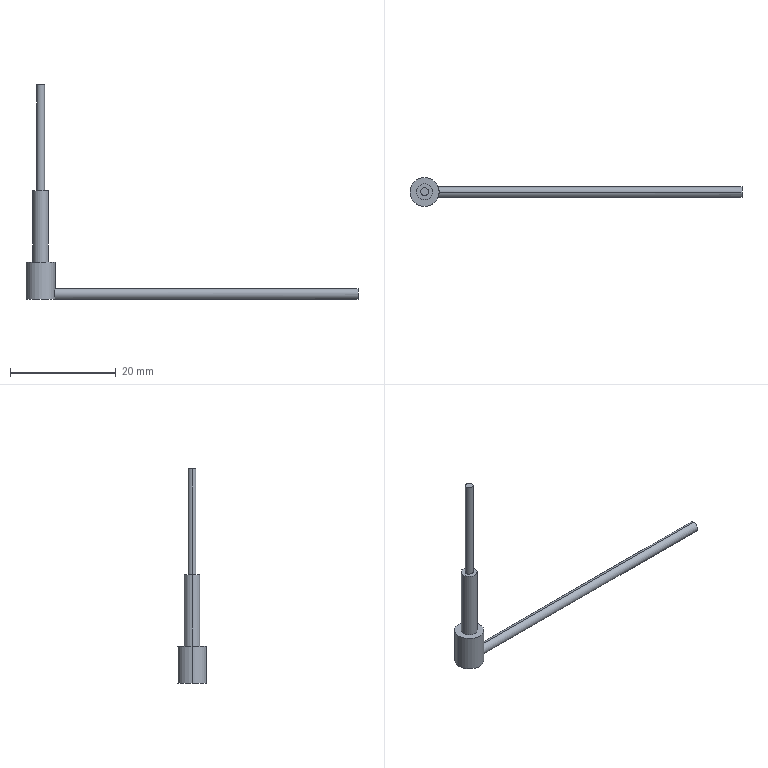Part | SolidWorks | features BaseBody 2 | 2 solids | 14 faces | box 62.75 x 5.5 x 40.5 mm | volume 476.928 mm3 | cylinder 8 | plane 6 | commonest cylinder face diameters 1.5 x2 2 x2 3 x2 5.5 x2
STEP:
#1=CARTESIAN_POINT('',(-0.75,0.,20.5));
#2=VERTEX_POINT('',#1);
#3=CARTESIAN_POINT('',(0.75,0.,20.5));
#4=VERTEX_POINT('',#3);
#5=CARTESIAN_POINT('',(0.,0.,20.5));
#6=DIRECTION('',(0.,0.,1.));
#7=DIRECTION('',(1.,0.,0.));
#8=AXIS2_PLACEMENT_3D('',#5,#6,#7);
#9=CIRCLE('',#8,0.75);
#10=EDGE_CURVE('',#2,#4,#9,.T.);
#11=ORIENTED_EDGE('',*,*,#10,.F.);
#12=CARTESIAN_POINT('',(0.,0.,20.5));
#13=DIRECTION('',(0.,0.,1.));
#14=DIRECTION('',(1.,0.,0.));
#15=AXIS2_PLACEMENT_3D('',#12,#13,#14);
#16=CIRCLE('',#15,0.75);
#17=EDGE_CURVE('',#4,#2,#16,.T.);
#18=ORIENTED_EDGE('',*,*,#17,.F.);
#19=EDGE_LOOP('',(#11,#18));
#20=FACE_OUTER_BOUND('',#19,.T.);
#21=CARTESIAN_POINT('',(0.,0.,20.5));
#22=DIRECTION('',(0.,0.,1.));
#23=DIRECTION('',(1.,0.,0.));
#24=AXIS2_PLACEMENT_3D('',#21,#22,#23);
#25=PLANE('',#24);
#26=ADVANCED_FACE('',(#20),#25,.F.);
#27=CARTESIAN_POINT('',(-0.75,0.,40.5));
#28=VERTEX_POINT('',#27);
#29=CARTESIAN_POINT('',(0.75,0.,40.5));
#30=VERTEX_POINT('',#29);
#31=CARTESIAN_POINT('',(0.,0.,40.5));
#32=DIRECTION('',(0.,0.,1.));
#33=DIRECTION('',(1.,0.,0.));
#34=AXIS2_PLACEMENT_3D('',#31,#32,#33);
#35=CIRCLE('',#34,0.75);
#36=EDGE_CURVE('',#28,#30,#35,.T.);
#37=ORIENTED_EDGE('',*,*,#36,.T.);
#38=CARTESIAN_POINT('',(0.,0.,40.5));
#39=DIRECTION('',(0.,0.,1.));
#40=DIRECTION('',(1.,0.,0.));
#41=AXIS2_PLACEMENT_3D('',#38,#39,#40);
#42=CIRCLE('',#41,0.75);
#43=EDGE_CURVE('',#30,#28,#42,.T.);
#44=ORIENTED_EDGE('',*,*,#43,.T.);
#45=EDGE_LOOP('',(#37,#44));
#46=FACE_OUTER_BOUND('',#45,.T.);
#47=CARTESIAN_POINT('',(0.,0.,40.5));
#48=DIRECTION('',(0.,0.,1.));
#49=DIRECTION('',(1.,0.,0.));
#50=AXIS2_PLACEMENT_3D('',#47,#48,#49);
#51=PLANE('',#50);
#52=ADVANCED_FACE('',(#46),#51,.T.);
#53=CARTESIAN_POINT('',(0.75,0.,40.5));
#54=DIRECTION('',(0.,0.,-1.));
#55=VECTOR('',#54,1000.);
#56=LINE('',#53,#55);
#57=EDGE_CURVE('',#30,#4,#56,.T.);
#58=ORIENTED_EDGE('',*,*,#57,.F.);
#59=ORIENTED_EDGE('',*,*,#36,.F.);
#60=CARTESIAN_POINT('',(-0.75,0.,40.5));
#61=DIRECTION('',(0.,0.,-1.));
#62=VECTOR('',#61,1000.);
#63=LINE('',#60,#62);
#64=EDGE_CURVE('',#28,#2,#63,.T.);
#65=ORIENTED_EDGE('',*,*,#64,.T.);
#66=ORIENTED_EDGE('',*,*,#10,.T.);
#67=EDGE_LOOP('',(#58,#59,#65,#66));
#68=FACE_OUTER_BOUND('',#67,.T.);
#69=CARTESIAN_POINT('',(0.,0.,40.5));
#70=DIRECTION('',(0.,0.,-1.));
#71=DIRECTION('',(-1.,0.,0.));
#72=AXIS2_PLACEMENT_3D('',#69,#70,#71);
#73=CYLINDRICAL_SURFACE('',#72,0.75);
#74=ADVANCED_FACE('',(#68),#73,.T.);
#75=ORIENTED_EDGE('',*,*,#43,.F.);
#76=ORIENTED_EDGE('',*,*,#57,.T.);
#77=ORIENTED_EDGE('',*,*,#17,.T.);
#78=ORIENTED_EDGE('',*,*,#64,.F.);
#79=EDGE_LOOP('',(#75,#76,#77,#78));
#80=FACE_OUTER_BOUND('',#79,.T.);
#81=CARTESIAN_POINT('',(0.,0.,40.5));
#82=DIRECTION('',(0.,0.,-1.));
#83=DIRECTION('',(-1.,0.,0.));
#84=AXIS2_PLACEMENT_3D('',#81,#82,#83);
#85=CYLINDRICAL_SURFACE('',#84,0.75);
#86=ADVANCED_FACE('',(#80),#85,.T.);
#87=CLOSED_SHELL('',(#26,#52,#74,#86));
#88=MANIFOLD_SOLID_BREP('',#87);
#89=CARTESIAN_POINT('',(60.,0.,2.));
#90=VERTEX_POINT('',#89);
#91=CARTESIAN_POINT('',(60.,0.,0.));
#92=VERTEX_POINT('',#91);
#93=CARTESIAN_POINT('',(60.,0.,1.));
#94=DIRECTION('',(1.,0.,0.));
#95=DIRECTION('',(0.,0.,-1.));
#96=AXIS2_PLACEMENT_3D('',#93,#94,#95);
#97=CIRCLE('',#96,1.);
#98=EDGE_CURVE('',#90,#92,#97,.T.);
#99=ORIENTED_EDGE('',*,*,#98,.T.);
#100=CARTESIAN_POINT('',(60.,0.,1.));
#101=DIRECTION('',(1.,0.,0.));
#102=DIRECTION('',(0.,0.,-1.));
#103=AXIS2_PLACEMENT_3D('',#100,#101,#102);
#104=CIRCLE('',#103,1.);
#105=EDGE_CURVE('',#92,#90,#104,.T.);
#106=ORIENTED_EDGE('',*,*,#105,.T.);
#107=EDGE_LOOP('',(#99,#106));
#108=FACE_OUTER_BOUND('',#107,.T.);
#109=CARTESIAN_POINT('',(60.,0.,1.));
#110=DIRECTION('',(1.,0.,0.));
#111=DIRECTION('',(0.,1.,0.));
#112=AXIS2_PLACEMENT_3D('',#109,#110,#111);
#113=PLANE('',#112);
#114=ADVANCED_FACE('',(#108),#113,.T.);
#115=CARTESIAN_POINT('',(2.75,0.,0.));
#116=VERTEX_POINT('',#115);
#117=CARTESIAN_POINT('',(60.,0.,0.));
#118=DIRECTION('',(-1.,0.,0.));
#119=VECTOR('',#118,1000.);
#120=LINE('',#117,#119);
#121=EDGE_CURVE('',#92,#116,#120,.T.);
#122=ORIENTED_EDGE('',*,*,#121,.F.);
#123=ORIENTED_EDGE('',*,*,#98,.F.);
#124=CARTESIAN_POINT('',(2.75,0.,2.));
#125=VERTEX_POINT('',#124);
#126=CARTESIAN_POINT('',(60.,0.,2.));
#127=DIRECTION('',(-1.,0.,0.));
#128=VECTOR('',#127,1000.);
#129=LINE('',#126,#128);
#130=EDGE_CURVE('',#90,#125,#129,.T.);
#131=ORIENTED_EDGE('',*,*,#130,.T.);
#132=CARTESIAN_POINT('',(2.75,0.,2.));
#133=CARTESIAN_POINT('',(2.75,-0.0625,2.));
#134=CARTESIAN_POINT('',(2.748,-0.1267,1.994));
#135=CARTESIAN_POINT('',(2.741,-0.2236,1.975));
#136=CARTESIAN_POINT('',(2.738,-0.256,1.967));
#137=CARTESIAN_POINT('',(2.733,-0.3044,1.953));
#138=CARTESIAN_POINT('',(2.73,-0.3286,1.945));
#139=CARTESIAN_POINT('',(2.727,-0.3567,1.934));
#140=CARTESIAN_POINT('',(2.725,-0.3687,1.93));
#141=CARTESIAN_POINT('',(2.724,-0.3767,1.926));
#142=CARTESIAN_POINT('',(2.723,-0.382,1.924));
#143=CARTESIAN_POINT('',(2.717,-0.4276,1.905));
#144=CARTESIAN_POINT('',(2.708,-0.478,1.881));
#145=CARTESIAN_POINT('',(2.692,-0.5607,1.829));
#146=CARTESIAN_POINT('',(2.686,-0.5895,1.809));
#147=CARTESIAN_POINT('',(2.676,-0.6334,1.774));
#148=CARTESIAN_POINT('',(2.672,-0.6481,1.762));
#149=CARTESIAN_POINT('',(2.665,-0.6778,1.736));
#150=CARTESIAN_POINT('',(2.662,-0.6917,1.723));
#151=CARTESIAN_POINT('',(2.641,-0.7708,1.643));
#152=CARTESIAN_POINT('',(2.628,-0.8127,1.585));
#153=CARTESIAN_POINT('',(2.616,-0.8483,1.53));
#154=CARTESIAN_POINT('',(2.614,-0.8546,1.519));
#155=CARTESIAN_POINT('',(2.612,-0.8615,1.508));
#156=CARTESIAN_POINT('',(2.611,-0.8629,1.505));
#157=CARTESIAN_POINT('',(2.61,-0.8655,1.501));
#158=CARTESIAN_POINT('',(2.61,-0.8676,1.497));
#159=CARTESIAN_POINT('',(2.607,-0.874,1.486));
#160=CARTESIAN_POINT('',(2.603,-0.8863,1.464));
#161=CARTESIAN_POINT('',(2.599,-0.8974,1.442));
#162=CARTESIAN_POINT('',(2.595,-0.9111,1.412));
#163=CARTESIAN_POINT('',(2.593,-0.9166,1.4));
#164=CARTESIAN_POINT('',(2.571,-0.9769,1.255));
#165=CARTESIAN_POINT('',(2.562,-1.,1.123));
#166=CARTESIAN_POINT('',(2.562,-1.,0.9379));
#167=CARTESIAN_POINT('',(2.564,-0.9942,0.8741));
#168=CARTESIAN_POINT('',(2.571,-0.9754,0.7773));
#169=CARTESIAN_POINT('',(2.574,-0.9675,0.7448));
#170=CARTESIAN_POINT('',(2.58,-0.9529,0.6961));
#171=CARTESIAN_POINT('',(2.583,-0.9449,0.6717));
#172=CARTESIAN_POINT('',(2.586,-0.9343,0.6434));
#173=CARTESIAN_POINT('',(2.588,-0.9296,0.6313));
#174=CARTESIAN_POINT('',(2.589,-0.9263,0.6232));
#175=CARTESIAN_POINT('',(2.59,-0.924,0.6176));
#176=CARTESIAN_POINT('',(2.596,-0.9069,0.5766));
#177=CARTESIAN_POINT('',(2.605,-0.8841,0.5281));
#178=CARTESIAN_POINT('',(2.621,-0.8326,0.4452));
#179=CARTESIAN_POINT('',(2.628,-0.8126,0.4159));
#180=CARTESIAN_POINT('',(2.638,-0.7772,0.3704));
#181=CARTESIAN_POINT('',(2.642,-0.7645,0.3551));
#182=CARTESIAN_POINT('',(2.649,-0.7372,0.3241));
#183=CARTESIAN_POINT('',(2.654,-0.7218,0.3076));
#184=CARTESIAN_POINT('',(2.673,-0.6478,0.2336));
#185=CARTESIAN_POINT('',(2.687,-0.588,0.1886));
#186=CARTESIAN_POINT('',(2.703,-0.5054,0.1365));
#187=CARTESIAN_POINT('',(2.708,-0.479,0.1218));
#188=CARTESIAN_POINT('',(2.714,-0.4417,0.1027));
#189=CARTESIAN_POINT('',(2.717,-0.4237,0.09403));
#190=CARTESIAN_POINT('',(2.72,-0.4037,0.08508));
#191=CARTESIAN_POINT('',(2.721,-0.3954,0.08149));
#192=CARTESIAN_POINT('',(2.722,-0.3899,0.07915));
#193=CARTESIAN_POINT('',(2.722,-0.3885,0.07855));
#194=CARTESIAN_POINT('',(2.741,-0.257,0.02376));
#195=CARTESIAN_POINT('',(2.75,-0.125,0.));
#196=CARTESIAN_POINT('',(2.75,0.,0.));
#197=B_SPLINE_CURVE_WITH_KNOTS('',3,(#132,#133,#134,#135,#136,#137,#138,#139,#140,#141,#142,#143,#144,#145,#146,#147,#148,#149,#150,#151,#152,#153,#154,#155,#156,#157,#158,#159,#160,#161,#162,#163,#164,#165,#166,#167,#168,#169,#170,#171,#172,#173,#174,#175,#176,#177,#178,#179,#180,#181,#182,#183,#184,#185,#186,#187,#188,#189,#190,#191,#192,#193,#194,#195,#196),.UNSPECIFIED.,.F.,.F.,(4,2,2,1,1,2,2,2,2,2,2,2,2,2,2,1,2,2,2,2,2,1,1,2,2,2,2,2,2,2,2,1,1,2,2,4),(0.,0.0625,0.09375,0.1094,0.1172,0.1211,0.125,0.1875,0.2187,0.2344,0.25,0.3125,0.3281,0.332,0.3359,0.3437,0.3594,0.375,0.5,0.5625,0.5937,0.6094,0.6172,0.6211,0.625,0.6875,0.7187,0.7344,0.75,0.8125,0.8437,0.8594,0.8672,0.8711,0.875,1.),.UNSPECIFIED.);
#198=EDGE_CURVE('',#125,#116,#197,.T.);
#199=ORIENTED_EDGE('',*,*,#198,.T.);
#200=EDGE_LOOP('',(#122,#123,#131,#199));
#201=FACE_OUTER_BOUND('',#200,.T.);
#202=CARTESIAN_POINT('',(60.,0.,1.));
#203=DIRECTION('',(-1.,0.,0.));
#204=DIRECTION('',(0.,0.,1.));
#205=AXIS2_PLACEMENT_3D('',#202,#203,#204);
#206=CYLINDRICAL_SURFACE('',#205,1.);
#207=ADVANCED_FACE('',(#201),#206,.T.);
#208=CARTESIAN_POINT('',(-1.5,0.,20.5));
#209=VERTEX_POINT('',#208);
#210=CARTESIAN_POINT('',(1.5,0.,20.5));
#211=VERTEX_POINT('',#210);
#212=CARTESIAN_POINT('',(0.,0.,20.5));
#213=DIRECTION('',(0.,0.,1.));
#214=DIRECTION('',(1.,0.,0.));
#215=AXIS2_PLACEMENT_3D('',#212,#213,#214);
#216=CIRCLE('',#215,1.5);
#217=EDGE_CURVE('',#209,#211,#216,.T.);
#218=ORIENTED_EDGE('',*,*,#217,.T.);
#219=CARTESIAN_POINT('',(0.,0.,20.5));
#220=DIRECTION('',(0.,0.,1.));
#221=DIRECTION('',(1.,0.,0.));
#222=AXIS2_PLACEMENT_3D('',#219,#220,#221);
#223=CIRCLE('',#222,1.5);
#224=EDGE_CURVE('',#211,#209,#223,.T.);
#225=ORIENTED_EDGE('',*,*,#224,.T.);
#226=EDGE_LOOP('',(#218,#225));
#227=FACE_OUTER_BOUND('',#226,.T.);
#228=CARTESIAN_POINT('',(0.,0.,20.5));
#229=DIRECTION('',(0.,0.,1.));
#230=DIRECTION('',(1.,0.,0.));
#231=AXIS2_PLACEMENT_3D('',#228,#229,#230);
#232=PLANE('',#231);
#233=ADVANCED_FACE('',(#227),#232,.T.);
#234=CARTESIAN_POINT('',(1.5,0.,7.));
#235=VERTEX_POINT('',#234);
#236=CARTESIAN_POINT('',(1.5,0.,20.5));
#237=DIRECTION('',(0.,0.,-1.));
#238=VECTOR('',#237,1000.);
#239=LINE('',#236,#238);
#240=EDGE_CURVE('',#211,#235,#239,.T.);
#241=ORIENTED_EDGE('',*,*,#240,.F.);
#242=ORIENTED_EDGE('',*,*,#217,.F.);
#243=CARTESIAN_POINT('',(-1.5,0.,7.));
#244=VERTEX_POINT('',#243);
#245=CARTESIAN_POINT('',(-1.5,0.,20.5));
#246=DIRECTION('',(0.,0.,-1.));
#247=VECTOR('',#246,1000.);
#248=LINE('',#245,#247);
#249=EDGE_CURVE('',#209,#244,#248,.T.);
#250=ORIENTED_EDGE('',*,*,#249,.T.);
#251=CARTESIAN_POINT('',(0.,0.,7.));
#252=DIRECTION('',(0.,0.,1.));
#253=DIRECTION('',(1.,0.,0.));
#254=AXIS2_PLACEMENT_3D('',#251,#252,#253);
#255=CIRCLE('',#254,1.5);
#256=EDGE_CURVE('',#244,#235,#255,.T.);
#257=ORIENTED_EDGE('',*,*,#256,.T.);
#258=EDGE_LOOP('',(#241,#242,#250,#257));
#259=FACE_OUTER_BOUND('',#258,.T.);
#260=CARTESIAN_POINT('',(0.,0.,20.5));
#261=DIRECTION('',(0.,0.,-1.));
#262=DIRECTION('',(-1.,0.,0.));
#263=AXIS2_PLACEMENT_3D('',#260,#261,#262);
#264=CYLINDRICAL_SURFACE('',#263,1.5);
#265=ADVANCED_FACE('',(#259),#264,.T.);
#266=CARTESIAN_POINT('',(-2.75,0.,0.));
#267=VERTEX_POINT('',#266);
#268=CARTESIAN_POINT('',(0.,0.,0.));
#269=DIRECTION('',(0.,0.,1.));
#270=DIRECTION('',(1.,0.,0.));
#271=AXIS2_PLACEMENT_3D('',#268,#269,#270);
#272=CIRCLE('',#271,2.75);
#273=EDGE_CURVE('',#116,#267,#272,.T.);
#274=ORIENTED_EDGE('',*,*,#273,.F.);
#275=CARTESIAN_POINT('',(0.,0.,0.));
#276=DIRECTION('',(0.,0.,1.));
#277=DIRECTION('',(1.,0.,0.));
#278=AXIS2_PLACEMENT_3D('',#275,#276,#277);
#279=CIRCLE('',#278,2.75);
#280=EDGE_CURVE('',#267,#116,#279,.T.);
#281=ORIENTED_EDGE('',*,*,#280,.F.);
#282=EDGE_LOOP('',(#274,#281));
#283=FACE_OUTER_BOUND('',#282,.T.);
#284=CARTESIAN_POINT('',(0.,0.,0.));
#285=DIRECTION('',(0.,0.,1.));
#286=DIRECTION('',(1.,0.,0.));
#287=AXIS2_PLACEMENT_3D('',#284,#285,#286);
#288=PLANE('',#287);
#289=ADVANCED_FACE('',(#283),#288,.F.);
#290=ORIENTED_EDGE('',*,*,#256,.F.);
#291=CARTESIAN_POINT('',(0.,0.,7.));
#292=DIRECTION('',(0.,0.,1.));
#293=DIRECTION('',(1.,0.,0.));
#294=AXIS2_PLACEMENT_3D('',#291,#292,#293);
#295=CIRCLE('',#294,1.5);
#296=EDGE_CURVE('',#235,#244,#295,.T.);
#297=ORIENTED_EDGE('',*,*,#296,.F.);
#298=EDGE_LOOP('',(#290,#297));
#299=FACE_BOUND('',#298,.T.);
#300=CARTESIAN_POINT('',(-2.75,0.,7.));
#301=VERTEX_POINT('',#300);
#302=CARTESIAN_POINT('',(2.75,0.,7.));
#303=VERTEX_POINT('',#302);
#304=CARTESIAN_POINT('',(0.,0.,7.));
#305=DIRECTION('',(0.,0.,1.));
#306=DIRECTION('',(1.,0.,0.));
#307=AXIS2_PLACEMENT_3D('',#304,#305,#306);
#308=CIRCLE('',#307,2.75);
#309=EDGE_CURVE('',#301,#303,#308,.T.);
#310=ORIENTED_EDGE('',*,*,#309,.T.);
#311=CARTESIAN_POINT('',(0.,0.,7.));
#312=DIRECTION('',(0.,0.,1.));
#313=DIRECTION('',(1.,0.,0.));
#314=AXIS2_PLACEMENT_3D('',#311,#312,#313);
#315=CIRCLE('',#314,2.75);
#316=EDGE_CURVE('',#303,#301,#315,.T.);
#317=ORIENTED_EDGE('',*,*,#316,.T.);
#318=EDGE_LOOP('',(#310,#317));
#319=FACE_OUTER_BOUND('',#318,.T.);
#320=CARTESIAN_POINT('',(0.,0.,7.));
#321=DIRECTION('',(0.,0.,1.));
#322=DIRECTION('',(1.,0.,0.));
#323=AXIS2_PLACEMENT_3D('',#320,#321,#322);
#324=PLANE('',#323);
#325=ADVANCED_FACE('',(#299,#319),#324,.T.);
#326=CARTESIAN_POINT('',(2.75,0.,7.));
#327=DIRECTION('',(0.,0.,-1.));
#328=VECTOR('',#327,1000.);
#329=LINE('',#326,#328);
#330=EDGE_CURVE('',#303,#125,#329,.T.);
#331=ORIENTED_EDGE('',*,*,#330,.F.);
#332=ORIENTED_EDGE('',*,*,#309,.F.);
#333=CARTESIAN_POINT('',(-2.75,0.,7.));
#334=DIRECTION('',(0.,0.,-1.));
#335=VECTOR('',#334,1000.);
#336=LINE('',#333,#335);
#337=EDGE_CURVE('',#301,#267,#336,.T.);
#338=ORIENTED_EDGE('',*,*,#337,.T.);
#339=ORIENTED_EDGE('',*,*,#280,.T.);
#340=ORIENTED_EDGE('',*,*,#198,.F.);
#341=EDGE_LOOP('',(#331,#332,#338,#339,#340));
#342=FACE_OUTER_BOUND('',#341,.T.);
#343=CARTESIAN_POINT('',(0.,0.,7.));
#344=DIRECTION('',(0.,0.,-1.));
#345=DIRECTION('',(-1.,0.,0.));
#346=AXIS2_PLACEMENT_3D('',#343,#344,#345);
#347=CYLINDRICAL_SURFACE('',#346,2.75);
#348=ADVANCED_FACE('',(#342),#347,.T.);
#349=ORIENTED_EDGE('',*,*,#316,.F.);
#350=ORIENTED_EDGE('',*,*,#330,.T.);
#351=CARTESIAN_POINT('',(2.75,0.,0.));
#352=CARTESIAN_POINT('',(2.75,0.06255,0.));
#353=CARTESIAN_POINT('',(2.748,0.1268,0.005887));
#354=CARTESIAN_POINT('',(2.741,0.2238,0.02481));
#355=CARTESIAN_POINT('',(2.738,0.2562,0.03279));
#356=CARTESIAN_POINT('',(2.733,0.3047,0.04741));
#357=CARTESIAN_POINT('',(2.73,0.3289,0.05537));
#358=CARTESIAN_POINT('',(2.727,0.357,0.06584));
#359=CARTESIAN_POINT('',(2.725,0.3691,0.07059));
#360=CARTESIAN_POINT('',(2.724,0.3771,0.0738));
#361=CARTESIAN_POINT('',(2.723,0.3824,0.07599));
#362=CARTESIAN_POINT('',(2.717,0.4279,0.09498));
#363=CARTESIAN_POINT('',(2.708,0.4783,0.1194));
#364=CARTESIAN_POINT('',(2.692,0.5609,0.1715));
#365=CARTESIAN_POINT('',(2.686,0.5896,0.1914));
#366=CARTESIAN_POINT('',(2.673,0.6481,0.2375));
#367=CARTESIAN_POINT('',(2.666,0.6763,0.2621));
#368=CARTESIAN_POINT('',(2.641,0.7698,0.3557));
#369=CARTESIAN_POINT('',(2.627,0.8156,0.4178));
#370=CARTESIAN_POINT('',(2.61,0.867,0.5006));
#371=CARTESIAN_POINT('',(2.605,0.8813,0.5266));
#372=CARTESIAN_POINT('',(2.599,0.8993,0.5624));
#373=CARTESIAN_POINT('',(2.596,0.9074,0.5795));
#374=CARTESIAN_POINT('',(2.593,0.9156,0.5979));
#375=CARTESIAN_POINT('',(2.592,0.9189,0.6055));
#376=CARTESIAN_POINT('',(2.591,0.921,0.6105));
#377=CARTESIAN_POINT('',(2.591,0.9214,0.6113));
#378=CARTESIAN_POINT('',(2.571,0.9767,0.7441));
#379=CARTESIAN_POINT('',(2.562,0.9999,0.8758));
#380=CARTESIAN_POINT('',(2.562,1.,1.061));
#381=CARTESIAN_POINT('',(2.564,0.9943,1.125));
#382=CARTESIAN_POINT('',(2.571,0.9756,1.222));
#383=CARTESIAN_POINT('',(2.574,0.9676,1.255));
#384=CARTESIAN_POINT('',(2.58,0.953,1.303));
#385=CARTESIAN_POINT('',(2.582,0.9477,1.32));
#386=CARTESIAN_POINT('',(2.586,0.9361,1.352));
#387=CARTESIAN_POINT('',(2.588,0.929,1.37));
#388=CARTESIAN_POINT('',(2.595,0.9113,1.413));
#389=CARTESIAN_POINT('',(2.599,0.8976,1.442));
#390=CARTESIAN_POINT('',(2.606,0.8776,1.479));
#391=CARTESIAN_POINT('',(2.608,0.8735,1.487));
#392=CARTESIAN_POINT('',(2.61,0.8671,1.498));
#393=CARTESIAN_POINT('',(2.61,0.8649,1.502));
#394=CARTESIAN_POINT('',(2.611,0.8623,1.506));
#395=CARTESIAN_POINT('',(2.614,0.8556,1.518));
#396=CARTESIAN_POINT('',(2.616,0.8478,1.53));
#397=CARTESIAN_POINT('',(2.623,0.8265,1.564));
#398=CARTESIAN_POINT('',(2.629,0.8089,1.589));
#399=CARTESIAN_POINT('',(2.638,0.7759,1.631));
#400=CARTESIAN_POINT('',(2.642,0.7638,1.646));
#401=CARTESIAN_POINT('',(2.649,0.7372,1.676));
#402=CARTESIAN_POINT('',(2.654,0.7216,1.693));
#403=CARTESIAN_POINT('',(2.673,0.6477,1.767));
#404=CARTESIAN_POINT('',(2.687,0.5879,1.812));
#405=CARTESIAN_POINT('',(2.703,0.5053,1.864));
#406=CARTESIAN_POINT('',(2.708,0.4789,1.878));
#407=CARTESIAN_POINT('',(2.714,0.4416,1.897));
#408=CARTESIAN_POINT('',(2.717,0.4235,1.906));
#409=CARTESIAN_POINT('',(2.72,0.4035,1.915));
#410=CARTESIAN_POINT('',(2.721,0.3952,1.919));
#411=CARTESIAN_POINT('',(2.722,0.3897,1.921));
#412=CARTESIAN_POINT('',(2.722,0.3883,1.922));
#413=CARTESIAN_POINT('',(2.741,0.2569,1.976));
#414=CARTESIAN_POINT('',(2.75,0.1249,2.));
#415=CARTESIAN_POINT('',(2.75,0.,2.));
#416=B_SPLINE_CURVE_WITH_KNOTS('',3,(#351,#352,#353,#354,#355,#356,#357,#358,#359,#360,#361,#362,#363,#364,#365,#366,#367,#368,#369,#370,#371,#372,#373,#374,#375,#376,#377,#378,#379,#380,#381,#382,#383,#384,#385,#386,#387,#388,#389,#390,#391,#392,#393,#394,#395,#396,#397,#398,#399,#400,#401,#402,#403,#404,#405,#406,#407,#408,#409,#410,#411,#412,#413,#414,#415),.UNSPECIFIED.,.F.,.F.,(4,2,2,1,1,2,2,2,2,2,2,2,1,1,2,2,2,2,2,2,2,2,2,2,1,2,2,2,2,2,2,1,1,2,2,4),(0.,0.0625,0.09375,0.1094,0.1172,0.1211,0.125,0.1875,0.2188,0.25,0.3125,0.3437,0.3594,0.3672,0.3711,0.375,0.5,0.5625,0.5938,0.6094,0.625,0.6563,0.6641,0.668,0.6719,0.6875,0.7188,0.7344,0.75,0.8125,0.8438,0.8594,0.8672,0.8711,0.875,1.),.UNSPECIFIED.);
#417=EDGE_CURVE('',#116,#125,#416,.T.);
#418=ORIENTED_EDGE('',*,*,#417,.F.);
#419=ORIENTED_EDGE('',*,*,#273,.T.);
#420=ORIENTED_EDGE('',*,*,#337,.F.);
#421=EDGE_LOOP('',(#349,#350,#418,#419,#420));
#422=FACE_OUTER_BOUND('',#421,.T.);
#423=CARTESIAN_POINT('',(0.,0.,7.));
#424=DIRECTION('',(0.,0.,-1.));
#425=DIRECTION('',(-1.,0.,0.));
#426=AXIS2_PLACEMENT_3D('',#423,#424,#425);
#427=CYLINDRICAL_SURFACE('',#426,2.75);
#428=ADVANCED_FACE('',(#422),#427,.T.);
#429=ORIENTED_EDGE('',*,*,#224,.F.);
#430=ORIENTED_EDGE('',*,*,#240,.T.);
#431=ORIENTED_EDGE('',*,*,#296,.T.);
#432=ORIENTED_EDGE('',*,*,#249,.F.);
#433=EDGE_LOOP('',(#429,#430,#431,#432));
#434=FACE_OUTER_BOUND('',#433,.T.);
#435=CARTESIAN_POINT('',(0.,0.,20.5));
#436=DIRECTION('',(0.,0.,-1.));
#437=DIRECTION('',(-1.,0.,0.));
#438=AXIS2_PLACEMENT_3D('',#435,#436,#437);
#439=CYLINDRICAL_SURFACE('',#438,1.5);
#440=ADVANCED_FACE('',(#434),#439,.T.);
#441=ORIENTED_EDGE('',*,*,#105,.F.);
#442=ORIENTED_EDGE('',*,*,#121,.T.);
#443=ORIENTED_EDGE('',*,*,#417,.T.);
#444=ORIENTED_EDGE('',*,*,#130,.F.);
#445=EDGE_LOOP('',(#441,#442,#443,#444));
#446=FACE_OUTER_BOUND('',#445,.T.);
#447=CARTESIAN_POINT('',(60.,0.,1.));
#448=DIRECTION('',(-1.,0.,0.));
#449=DIRECTION('',(0.,0.,1.));
#450=AXIS2_PLACEMENT_3D('',#447,#448,#449);
#451=CYLINDRICAL_SURFACE('',#450,1.);
#452=ADVANCED_FACE('',(#446),#451,.T.);
#453=CLOSED_SHELL('',(#114,#207,#233,#265,#289,#325,#348,#428,#440,#452));
#454=MANIFOLD_SOLID_BREP('',#453);
#455=CARTESIAN_POINT('',(0.,0.,0.));
#456=DIRECTION('',(0.,0.,1.));
#457=DIRECTION('',(1.,0.,0.));
#458=AXIS2_PLACEMENT_3D('',#455,#456,#457);
#459=(LENGTH_UNIT()NAMED_UNIT(*)SI_UNIT(.MILLI.,.METRE.));
#460=UNCERTAINTY_MEASURE_WITH_UNIT(LENGTH_MEASURE(0.00001),#459,'','');
#461=(NAMED_UNIT(*)PLANE_ANGLE_UNIT()SI_UNIT($,.RADIAN.));
#462=(NAMED_UNIT(*)SI_UNIT($,.STERADIAN.)SOLID_ANGLE_UNIT());
#463=(GEOMETRIC_REPRESENTATION_CONTEXT(3)GLOBAL_UNCERTAINTY_ASSIGNED_CONTEXT((#460))GLOBAL_UNIT_ASSIGNED_CONTEXT((#459,#461,#462))REPRESENTATION_CONTEXT('',''));
#464=ADVANCED_BREP_SHAPE_REPRESENTATION('',(#88,#454,#458),#463);